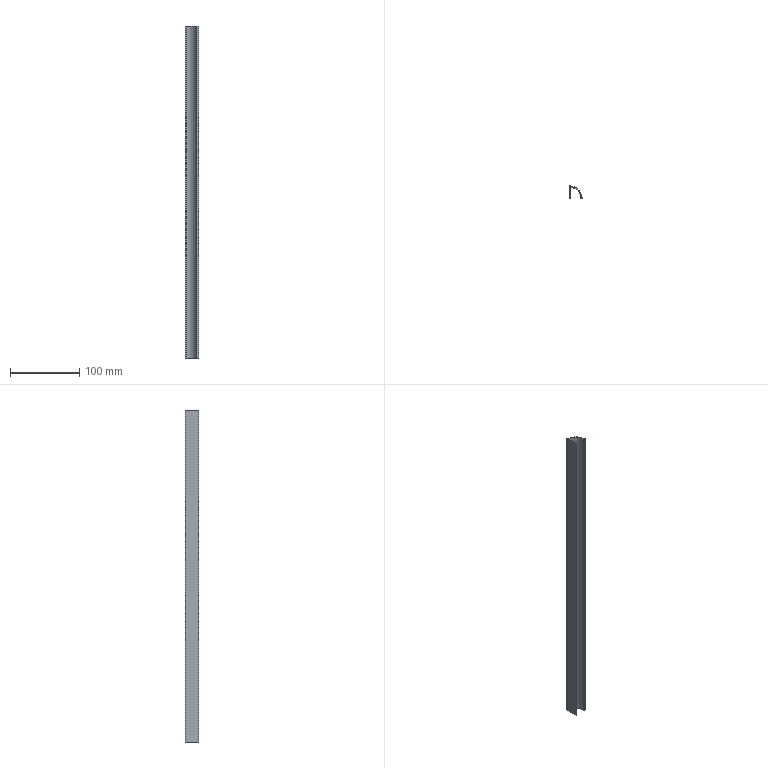Part | SolidWorks | features Extrusion 1 | 1 solid | 19 faces | box 19 x 19 x 480 mm | volume 26207 mm3 | plane 17 | cylinder 2 | commonest cylinder face diameters 30 x1 32 x1
STEP:
#1=CARTESIAN_POINT('',(0.,0.,0.));
#2=VERTEX_POINT('',#1);
#3=CARTESIAN_POINT('',(1.5,0.,0.));
#4=VERTEX_POINT('',#3);
#5=CARTESIAN_POINT('',(0.,0.,0.));
#6=DIRECTION('',(1.,0.,0.));
#7=VECTOR('',#6,1000.);
#8=LINE('',#5,#7);
#9=EDGE_CURVE('',#2,#4,#8,.T.);
#10=ORIENTED_EDGE('',*,*,#9,.T.);
#11=CARTESIAN_POINT('',(1.5,0.,480.));
#12=VERTEX_POINT('',#11);
#13=CARTESIAN_POINT('',(1.5,0.,480.));
#14=DIRECTION('',(0.,0.,-1.));
#15=VECTOR('',#14,1000.);
#16=LINE('',#13,#15);
#17=EDGE_CURVE('',#12,#4,#16,.T.);
#18=ORIENTED_EDGE('',*,*,#17,.F.);
#19=CARTESIAN_POINT('',(0.,0.,480.));
#20=VERTEX_POINT('',#19);
#21=CARTESIAN_POINT('',(0.,0.,480.));
#22=DIRECTION('',(1.,0.,0.));
#23=VECTOR('',#22,1000.);
#24=LINE('',#21,#23);
#25=EDGE_CURVE('',#20,#12,#24,.T.);
#26=ORIENTED_EDGE('',*,*,#25,.F.);
#27=CARTESIAN_POINT('',(0.,0.,480.));
#28=DIRECTION('',(0.,0.,-1.));
#29=VECTOR('',#28,1000.);
#30=LINE('',#27,#29);
#31=EDGE_CURVE('',#20,#2,#30,.T.);
#32=ORIENTED_EDGE('',*,*,#31,.T.);
#33=EDGE_LOOP('',(#10,#18,#26,#32));
#34=FACE_OUTER_BOUND('',#33,.T.);
#35=CARTESIAN_POINT('',(0.,0.,480.));
#36=DIRECTION('',(0.,1.,0.));
#37=DIRECTION('',(0.,0.,1.));
#38=AXIS2_PLACEMENT_3D('',#35,#36,#37);
#39=PLANE('',#38);
#40=ADVANCED_FACE('',(#34),#39,.F.);
#41=CARTESIAN_POINT('',(1.5,16.5,0.));
#42=VERTEX_POINT('',#41);
#43=CARTESIAN_POINT('',(1.5,0.,0.));
#44=DIRECTION('',(0.,1.,0.));
#45=VECTOR('',#44,1000.);
#46=LINE('',#43,#45);
#47=EDGE_CURVE('',#4,#42,#46,.T.);
#48=ORIENTED_EDGE('',*,*,#47,.T.);
#49=CARTESIAN_POINT('',(1.5,16.5,480.));
#50=VERTEX_POINT('',#49);
#51=CARTESIAN_POINT('',(1.5,16.5,480.));
#52=DIRECTION('',(0.,0.,-1.));
#53=VECTOR('',#52,1000.);
#54=LINE('',#51,#53);
#55=EDGE_CURVE('',#50,#42,#54,.T.);
#56=ORIENTED_EDGE('',*,*,#55,.F.);
#57=CARTESIAN_POINT('',(1.5,0.,480.));
#58=DIRECTION('',(0.,1.,0.));
#59=VECTOR('',#58,1000.);
#60=LINE('',#57,#59);
#61=EDGE_CURVE('',#12,#50,#60,.T.);
#62=ORIENTED_EDGE('',*,*,#61,.F.);
#63=ORIENTED_EDGE('',*,*,#17,.T.);
#64=EDGE_LOOP('',(#48,#56,#62,#63));
#65=FACE_OUTER_BOUND('',#64,.T.);
#66=CARTESIAN_POINT('',(1.5,0.,480.));
#67=DIRECTION('',(-1.,0.,0.));
#68=DIRECTION('',(0.,0.,1.));
#69=AXIS2_PLACEMENT_3D('',#66,#67,#68);
#70=PLANE('',#69);
#71=ADVANCED_FACE('',(#65),#70,.F.);
#72=CARTESIAN_POINT('',(16.5,1.5,0.));
#73=VERTEX_POINT('',#72);
#74=CARTESIAN_POINT('',(1.5,1.5,0.));
#75=DIRECTION('',(0.,0.,-1.));
#76=DIRECTION('',(-1.,0.,0.));
#77=AXIS2_PLACEMENT_3D('',#74,#75,#76);
#78=CIRCLE('',#77,15.);
#79=EDGE_CURVE('',#42,#73,#78,.T.);
#80=ORIENTED_EDGE('',*,*,#79,.T.);
#81=CARTESIAN_POINT('',(16.5,1.5,480.));
#82=VERTEX_POINT('',#81);
#83=CARTESIAN_POINT('',(16.5,1.5,480.));
#84=DIRECTION('',(0.,0.,-1.));
#85=VECTOR('',#84,1000.);
#86=LINE('',#83,#85);
#87=EDGE_CURVE('',#82,#73,#86,.T.);
#88=ORIENTED_EDGE('',*,*,#87,.F.);
#89=CARTESIAN_POINT('',(1.5,1.5,480.));
#90=DIRECTION('',(0.,0.,-1.));
#91=DIRECTION('',(-1.,0.,0.));
#92=AXIS2_PLACEMENT_3D('',#89,#90,#91);
#93=CIRCLE('',#92,15.);
#94=EDGE_CURVE('',#50,#82,#93,.T.);
#95=ORIENTED_EDGE('',*,*,#94,.F.);
#96=ORIENTED_EDGE('',*,*,#55,.T.);
#97=EDGE_LOOP('',(#80,#88,#95,#96));
#98=FACE_OUTER_BOUND('',#97,.T.);
#99=CARTESIAN_POINT('',(1.5,1.5,480.));
#100=DIRECTION('',(0.,0.,-1.));
#101=DIRECTION('',(-1.,0.,0.));
#102=AXIS2_PLACEMENT_3D('',#99,#100,#101);
#103=CYLINDRICAL_SURFACE('',#102,15.);
#104=ADVANCED_FACE('',(#98),#103,.F.);
#105=CARTESIAN_POINT('',(16.5,0.,0.));
#106=VERTEX_POINT('',#105);
#107=CARTESIAN_POINT('',(16.5,1.5,0.));
#108=DIRECTION('',(0.,-1.,0.));
#109=VECTOR('',#108,1000.);
#110=LINE('',#107,#109);
#111=EDGE_CURVE('',#73,#106,#110,.T.);
#112=ORIENTED_EDGE('',*,*,#111,.T.);
#113=CARTESIAN_POINT('',(16.5,0.,480.));
#114=VERTEX_POINT('',#113);
#115=CARTESIAN_POINT('',(16.5,0.,480.));
#116=DIRECTION('',(0.,0.,-1.));
#117=VECTOR('',#116,1000.);
#118=LINE('',#115,#117);
#119=EDGE_CURVE('',#114,#106,#118,.T.);
#120=ORIENTED_EDGE('',*,*,#119,.F.);
#121=CARTESIAN_POINT('',(16.5,1.5,480.));
#122=DIRECTION('',(0.,-1.,0.));
#123=VECTOR('',#122,1000.);
#124=LINE('',#121,#123);
#125=EDGE_CURVE('',#82,#114,#124,.T.);
#126=ORIENTED_EDGE('',*,*,#125,.F.);
#127=ORIENTED_EDGE('',*,*,#87,.T.);
#128=EDGE_LOOP('',(#112,#120,#126,#127));
#129=FACE_OUTER_BOUND('',#128,.T.);
#130=CARTESIAN_POINT('',(16.5,1.5,480.));
#131=DIRECTION('',(1.,0.,0.));
#132=DIRECTION('',(0.,0.,-1.));
#133=AXIS2_PLACEMENT_3D('',#130,#131,#132);
#134=PLANE('',#133);
#135=ADVANCED_FACE('',(#129),#134,.F.);
#136=CARTESIAN_POINT('',(19.,0.,0.));
#137=VERTEX_POINT('',#136);
#138=CARTESIAN_POINT('',(16.5,0.,0.));
#139=DIRECTION('',(1.,0.,0.));
#140=VECTOR('',#139,1000.);
#141=LINE('',#138,#140);
#142=EDGE_CURVE('',#106,#137,#141,.T.);
#143=ORIENTED_EDGE('',*,*,#142,.T.);
#144=CARTESIAN_POINT('',(19.,0.,480.));
#145=VERTEX_POINT('',#144);
#146=CARTESIAN_POINT('',(19.,0.,480.));
#147=DIRECTION('',(0.,0.,-1.));
#148=VECTOR('',#147,1000.);
#149=LINE('',#146,#148);
#150=EDGE_CURVE('',#145,#137,#149,.T.);
#151=ORIENTED_EDGE('',*,*,#150,.F.);
#152=CARTESIAN_POINT('',(16.5,0.,480.));
#153=DIRECTION('',(1.,0.,0.));
#154=VECTOR('',#153,1000.);
#155=LINE('',#152,#154);
#156=EDGE_CURVE('',#114,#145,#155,.T.);
#157=ORIENTED_EDGE('',*,*,#156,.F.);
#158=ORIENTED_EDGE('',*,*,#119,.T.);
#159=EDGE_LOOP('',(#143,#151,#157,#158));
#160=FACE_OUTER_BOUND('',#159,.T.);
#161=CARTESIAN_POINT('',(16.5,0.,480.));
#162=DIRECTION('',(0.,1.,0.));
#163=DIRECTION('',(0.,0.,1.));
#164=AXIS2_PLACEMENT_3D('',#161,#162,#163);
#165=PLANE('',#164);
#166=ADVANCED_FACE('',(#160),#165,.F.);
#167=CARTESIAN_POINT('',(19.,1.5,0.));
#168=VERTEX_POINT('',#167);
#169=CARTESIAN_POINT('',(19.,0.,0.));
#170=DIRECTION('',(0.,1.,0.));
#171=VECTOR('',#170,1000.);
#172=LINE('',#169,#171);
#173=EDGE_CURVE('',#137,#168,#172,.T.);
#174=ORIENTED_EDGE('',*,*,#173,.T.);
#175=CARTESIAN_POINT('',(19.,1.5,480.));
#176=VERTEX_POINT('',#175);
#177=CARTESIAN_POINT('',(19.,1.5,480.));
#178=DIRECTION('',(0.,0.,-1.));
#179=VECTOR('',#178,1000.);
#180=LINE('',#177,#179);
#181=EDGE_CURVE('',#176,#168,#180,.T.);
#182=ORIENTED_EDGE('',*,*,#181,.F.);
#183=CARTESIAN_POINT('',(19.,0.,480.));
#184=DIRECTION('',(0.,1.,0.));
#185=VECTOR('',#184,1000.);
#186=LINE('',#183,#185);
#187=EDGE_CURVE('',#145,#176,#186,.T.);
#188=ORIENTED_EDGE('',*,*,#187,.F.);
#189=ORIENTED_EDGE('',*,*,#150,.T.);
#190=EDGE_LOOP('',(#174,#182,#188,#189));
#191=FACE_OUTER_BOUND('',#190,.T.);
#192=CARTESIAN_POINT('',(19.,0.,480.));
#193=DIRECTION('',(-1.,0.,0.));
#194=DIRECTION('',(0.,0.,1.));
#195=AXIS2_PLACEMENT_3D('',#192,#193,#194);
#196=PLANE('',#195);
#197=ADVANCED_FACE('',(#191),#196,.F.);
#198=CARTESIAN_POINT('',(18.5,1.5,0.));
#199=VERTEX_POINT('',#198);
#200=CARTESIAN_POINT('',(18.5,1.5,0.));
#201=DIRECTION('',(-1.,0.,0.));
#202=VECTOR('',#201,1000.);
#203=LINE('',#200,#202);
#204=EDGE_CURVE('',#168,#199,#203,.T.);
#205=ORIENTED_EDGE('',*,*,#204,.T.);
#206=CARTESIAN_POINT('',(18.5,1.5,480.));
#207=VERTEX_POINT('',#206);
#208=CARTESIAN_POINT('',(18.5,1.5,480.));
#209=DIRECTION('',(0.,0.,-1.));
#210=VECTOR('',#209,1000.);
#211=LINE('',#208,#210);
#212=EDGE_CURVE('',#207,#199,#211,.T.);
#213=ORIENTED_EDGE('',*,*,#212,.F.);
#214=CARTESIAN_POINT('',(18.5,1.5,480.));
#215=DIRECTION('',(-1.,0.,0.));
#216=VECTOR('',#215,1000.);
#217=LINE('',#214,#216);
#218=EDGE_CURVE('',#176,#207,#217,.T.);
#219=ORIENTED_EDGE('',*,*,#218,.F.);
#220=ORIENTED_EDGE('',*,*,#181,.T.);
#221=EDGE_LOOP('',(#205,#213,#219,#220));
#222=FACE_OUTER_BOUND('',#221,.T.);
#223=CARTESIAN_POINT('',(18.5,1.5,480.));
#224=DIRECTION('',(0.,-1.,0.));
#225=DIRECTION('',(0.,0.,-1.));
#226=AXIS2_PLACEMENT_3D('',#223,#224,#225);
#227=PLANE('',#226);
#228=ADVANCED_FACE('',(#222),#227,.F.);
#229=CARTESIAN_POINT('',(18.5,0.5,0.));
#230=VERTEX_POINT('',#229);
#231=CARTESIAN_POINT('',(18.5,0.5,0.));
#232=DIRECTION('',(0.,-1.,0.));
#233=VECTOR('',#232,1000.);
#234=LINE('',#231,#233);
#235=EDGE_CURVE('',#199,#230,#234,.T.);
#236=ORIENTED_EDGE('',*,*,#235,.T.);
#237=CARTESIAN_POINT('',(18.5,0.5,480.));
#238=VERTEX_POINT('',#237);
#239=CARTESIAN_POINT('',(18.5,0.5,480.));
#240=DIRECTION('',(0.,0.,-1.));
#241=VECTOR('',#240,1000.);
#242=LINE('',#239,#241);
#243=EDGE_CURVE('',#238,#230,#242,.T.);
#244=ORIENTED_EDGE('',*,*,#243,.F.);
#245=CARTESIAN_POINT('',(18.5,0.5,480.));
#246=DIRECTION('',(0.,-1.,0.));
#247=VECTOR('',#246,1000.);
#248=LINE('',#245,#247);
#249=EDGE_CURVE('',#207,#238,#248,.T.);
#250=ORIENTED_EDGE('',*,*,#249,.F.);
#251=ORIENTED_EDGE('',*,*,#212,.T.);
#252=EDGE_LOOP('',(#236,#244,#250,#251));
#253=FACE_OUTER_BOUND('',#252,.T.);
#254=CARTESIAN_POINT('',(18.5,0.5,480.));
#255=DIRECTION('',(1.,0.,0.));
#256=DIRECTION('',(0.,0.,-1.));
#257=AXIS2_PLACEMENT_3D('',#254,#255,#256);
#258=PLANE('',#257);
#259=ADVANCED_FACE('',(#253),#258,.F.);
#260=CARTESIAN_POINT('',(17.5,0.5,0.));
#261=VERTEX_POINT('',#260);
#262=CARTESIAN_POINT('',(17.5,0.5,0.));
#263=DIRECTION('',(-1.,0.,0.));
#264=VECTOR('',#263,1000.);
#265=LINE('',#262,#264);
#266=EDGE_CURVE('',#230,#261,#265,.T.);
#267=ORIENTED_EDGE('',*,*,#266,.T.);
#268=CARTESIAN_POINT('',(17.5,0.5,480.));
#269=VERTEX_POINT('',#268);
#270=CARTESIAN_POINT('',(17.5,0.5,480.));
#271=DIRECTION('',(0.,0.,-1.));
#272=VECTOR('',#271,1000.);
#273=LINE('',#270,#272);
#274=EDGE_CURVE('',#269,#261,#273,.T.);
#275=ORIENTED_EDGE('',*,*,#274,.F.);
#276=CARTESIAN_POINT('',(17.5,0.5,480.));
#277=DIRECTION('',(-1.,0.,0.));
#278=VECTOR('',#277,1000.);
#279=LINE('',#276,#278);
#280=EDGE_CURVE('',#238,#269,#279,.T.);
#281=ORIENTED_EDGE('',*,*,#280,.F.);
#282=ORIENTED_EDGE('',*,*,#243,.T.);
#283=EDGE_LOOP('',(#267,#275,#281,#282));
#284=FACE_OUTER_BOUND('',#283,.T.);
#285=CARTESIAN_POINT('',(17.5,0.5,480.));
#286=DIRECTION('',(0.,-1.,0.));
#287=DIRECTION('',(0.,0.,-1.));
#288=AXIS2_PLACEMENT_3D('',#285,#286,#287);
#289=PLANE('',#288);
#290=ADVANCED_FACE('',(#284),#289,.F.);
#291=CARTESIAN_POINT('',(17.5,1.5,0.));
#292=VERTEX_POINT('',#291);
#293=CARTESIAN_POINT('',(17.5,1.5,0.));
#294=DIRECTION('',(0.,1.,0.));
#295=VECTOR('',#294,1000.);
#296=LINE('',#293,#295);
#297=EDGE_CURVE('',#261,#292,#296,.T.);
#298=ORIENTED_EDGE('',*,*,#297,.T.);
#299=CARTESIAN_POINT('',(17.5,1.5,480.));
#300=VERTEX_POINT('',#299);
#301=CARTESIAN_POINT('',(17.5,1.5,480.));
#302=DIRECTION('',(0.,0.,-1.));
#303=VECTOR('',#302,1000.);
#304=LINE('',#301,#303);
#305=EDGE_CURVE('',#300,#292,#304,.T.);
#306=ORIENTED_EDGE('',*,*,#305,.F.);
#307=CARTESIAN_POINT('',(17.5,1.5,480.));
#308=DIRECTION('',(0.,1.,0.));
#309=VECTOR('',#308,1000.);
#310=LINE('',#307,#309);
#311=EDGE_CURVE('',#269,#300,#310,.T.);
#312=ORIENTED_EDGE('',*,*,#311,.F.);
#313=ORIENTED_EDGE('',*,*,#274,.T.);
#314=EDGE_LOOP('',(#298,#306,#312,#313));
#315=FACE_OUTER_BOUND('',#314,.T.);
#316=CARTESIAN_POINT('',(17.5,1.5,480.));
#317=DIRECTION('',(-1.,0.,0.));
#318=DIRECTION('',(0.,0.,1.));
#319=AXIS2_PLACEMENT_3D('',#316,#317,#318);
#320=PLANE('',#319);
#321=ADVANCED_FACE('',(#315),#320,.F.);
#322=CARTESIAN_POINT('',(1.5,17.5,0.));
#323=VERTEX_POINT('',#322);
#324=CARTESIAN_POINT('',(1.5,1.5,0.));
#325=DIRECTION('',(0.,0.,1.));
#326=DIRECTION('',(-1.,0.,0.));
#327=AXIS2_PLACEMENT_3D('',#324,#325,#326);
#328=CIRCLE('',#327,16.);
#329=EDGE_CURVE('',#292,#323,#328,.T.);
#330=ORIENTED_EDGE('',*,*,#329,.T.);
#331=CARTESIAN_POINT('',(1.5,17.5,480.));
#332=VERTEX_POINT('',#331);
#333=CARTESIAN_POINT('',(1.5,17.5,480.));
#334=DIRECTION('',(0.,0.,-1.));
#335=VECTOR('',#334,1000.);
#336=LINE('',#333,#335);
#337=EDGE_CURVE('',#332,#323,#336,.T.);
#338=ORIENTED_EDGE('',*,*,#337,.F.);
#339=CARTESIAN_POINT('',(1.5,1.5,480.));
#340=DIRECTION('',(0.,0.,1.));
#341=DIRECTION('',(-1.,0.,0.));
#342=AXIS2_PLACEMENT_3D('',#339,#340,#341);
#343=CIRCLE('',#342,16.);
#344=EDGE_CURVE('',#300,#332,#343,.T.);
#345=ORIENTED_EDGE('',*,*,#344,.F.);
#346=ORIENTED_EDGE('',*,*,#305,.T.);
#347=EDGE_LOOP('',(#330,#338,#345,#346));
#348=FACE_OUTER_BOUND('',#347,.T.);
#349=CARTESIAN_POINT('',(1.5,1.5,480.));
#350=DIRECTION('',(0.,0.,-1.));
#351=DIRECTION('',(-1.,0.,0.));
#352=AXIS2_PLACEMENT_3D('',#349,#350,#351);
#353=CYLINDRICAL_SURFACE('',#352,16.);
#354=ADVANCED_FACE('',(#348),#353,.T.);
#355=CARTESIAN_POINT('',(0.5,17.5,0.));
#356=VERTEX_POINT('',#355);
#357=CARTESIAN_POINT('',(0.5,17.5,0.));
#358=DIRECTION('',(-1.,0.,0.));
#359=VECTOR('',#358,1000.);
#360=LINE('',#357,#359);
#361=EDGE_CURVE('',#323,#356,#360,.T.);
#362=ORIENTED_EDGE('',*,*,#361,.T.);
#363=CARTESIAN_POINT('',(0.5,17.5,480.));
#364=VERTEX_POINT('',#363);
#365=CARTESIAN_POINT('',(0.5,17.5,480.));
#366=DIRECTION('',(0.,0.,-1.));
#367=VECTOR('',#366,1000.);
#368=LINE('',#365,#367);
#369=EDGE_CURVE('',#364,#356,#368,.T.);
#370=ORIENTED_EDGE('',*,*,#369,.F.);
#371=CARTESIAN_POINT('',(0.5,17.5,480.));
#372=DIRECTION('',(-1.,0.,0.));
#373=VECTOR('',#372,1000.);
#374=LINE('',#371,#373);
#375=EDGE_CURVE('',#332,#364,#374,.T.);
#376=ORIENTED_EDGE('',*,*,#375,.F.);
#377=ORIENTED_EDGE('',*,*,#337,.T.);
#378=EDGE_LOOP('',(#362,#370,#376,#377));
#379=FACE_OUTER_BOUND('',#378,.T.);
#380=CARTESIAN_POINT('',(0.5,17.5,480.));
#381=DIRECTION('',(0.,-1.,0.));
#382=DIRECTION('',(0.,0.,-1.));
#383=AXIS2_PLACEMENT_3D('',#380,#381,#382);
#384=PLANE('',#383);
#385=ADVANCED_FACE('',(#379),#384,.F.);
#386=CARTESIAN_POINT('',(0.5,18.5,0.));
#387=VERTEX_POINT('',#386);
#388=CARTESIAN_POINT('',(0.5,18.5,0.));
#389=DIRECTION('',(0.,1.,0.));
#390=VECTOR('',#389,1000.);
#391=LINE('',#388,#390);
#392=EDGE_CURVE('',#356,#387,#391,.T.);
#393=ORIENTED_EDGE('',*,*,#392,.T.);
#394=CARTESIAN_POINT('',(0.5,18.5,480.));
#395=VERTEX_POINT('',#394);
#396=CARTESIAN_POINT('',(0.5,18.5,480.));
#397=DIRECTION('',(0.,0.,-1.));
#398=VECTOR('',#397,1000.);
#399=LINE('',#396,#398);
#400=EDGE_CURVE('',#395,#387,#399,.T.);
#401=ORIENTED_EDGE('',*,*,#400,.F.);
#402=CARTESIAN_POINT('',(0.5,18.5,480.));
#403=DIRECTION('',(0.,1.,0.));
#404=VECTOR('',#403,1000.);
#405=LINE('',#402,#404);
#406=EDGE_CURVE('',#364,#395,#405,.T.);
#407=ORIENTED_EDGE('',*,*,#406,.F.);
#408=ORIENTED_EDGE('',*,*,#369,.T.);
#409=EDGE_LOOP('',(#393,#401,#407,#408));
#410=FACE_OUTER_BOUND('',#409,.T.);
#411=CARTESIAN_POINT('',(0.5,18.5,480.));
#412=DIRECTION('',(-1.,0.,0.));
#413=DIRECTION('',(0.,0.,1.));
#414=AXIS2_PLACEMENT_3D('',#411,#412,#413);
#415=PLANE('',#414);
#416=ADVANCED_FACE('',(#410),#415,.F.);
#417=CARTESIAN_POINT('',(1.5,18.5,0.));
#418=VERTEX_POINT('',#417);
#419=CARTESIAN_POINT('',(1.5,18.5,0.));
#420=DIRECTION('',(1.,0.,0.));
#421=VECTOR('',#420,1000.);
#422=LINE('',#419,#421);
#423=EDGE_CURVE('',#387,#418,#422,.T.);
#424=ORIENTED_EDGE('',*,*,#423,.T.);
#425=CARTESIAN_POINT('',(1.5,18.5,480.));
#426=VERTEX_POINT('',#425);
#427=CARTESIAN_POINT('',(1.5,18.5,480.));
#428=DIRECTION('',(0.,0.,-1.));
#429=VECTOR('',#428,1000.);
#430=LINE('',#427,#429);
#431=EDGE_CURVE('',#426,#418,#430,.T.);
#432=ORIENTED_EDGE('',*,*,#431,.F.);
#433=CARTESIAN_POINT('',(1.5,18.5,480.));
#434=DIRECTION('',(1.,0.,0.));
#435=VECTOR('',#434,1000.);
#436=LINE('',#433,#435);
#437=EDGE_CURVE('',#395,#426,#436,.T.);
#438=ORIENTED_EDGE('',*,*,#437,.F.);
#439=ORIENTED_EDGE('',*,*,#400,.T.);
#440=EDGE_LOOP('',(#424,#432,#438,#439));
#441=FACE_OUTER_BOUND('',#440,.T.);
#442=CARTESIAN_POINT('',(1.5,18.5,480.));
#443=DIRECTION('',(0.,1.,0.));
#444=DIRECTION('',(0.,0.,1.));
#445=AXIS2_PLACEMENT_3D('',#442,#443,#444);
#446=PLANE('',#445);
#447=ADVANCED_FACE('',(#441),#446,.F.);
#448=CARTESIAN_POINT('',(1.5,19.,0.));
#449=VERTEX_POINT('',#448);
#450=CARTESIAN_POINT('',(1.5,19.,0.));
#451=DIRECTION('',(0.,1.,0.));
#452=VECTOR('',#451,1000.);
#453=LINE('',#450,#452);
#454=EDGE_CURVE('',#418,#449,#453,.T.);
#455=ORIENTED_EDGE('',*,*,#454,.T.);
#456=CARTESIAN_POINT('',(1.5,19.,480.));
#457=VERTEX_POINT('',#456);
#458=CARTESIAN_POINT('',(1.5,19.,480.));
#459=DIRECTION('',(0.,0.,-1.));
#460=VECTOR('',#459,1000.);
#461=LINE('',#458,#460);
#462=EDGE_CURVE('',#457,#449,#461,.T.);
#463=ORIENTED_EDGE('',*,*,#462,.F.);
#464=CARTESIAN_POINT('',(1.5,19.,480.));
#465=DIRECTION('',(0.,1.,0.));
#466=VECTOR('',#465,1000.);
#467=LINE('',#464,#466);
#468=EDGE_CURVE('',#426,#457,#467,.T.);
#469=ORIENTED_EDGE('',*,*,#468,.F.);
#470=ORIENTED_EDGE('',*,*,#431,.T.);
#471=EDGE_LOOP('',(#455,#463,#469,#470));
#472=FACE_OUTER_BOUND('',#471,.T.);
#473=CARTESIAN_POINT('',(1.5,19.,480.));
#474=DIRECTION('',(-1.,0.,0.));
#475=DIRECTION('',(0.,0.,1.));
#476=AXIS2_PLACEMENT_3D('',#473,#474,#475);
#477=PLANE('',#476);
#478=ADVANCED_FACE('',(#472),#477,.F.);
#479=CARTESIAN_POINT('',(0.,19.,0.));
#480=VERTEX_POINT('',#479);
#481=CARTESIAN_POINT('',(0.,19.,0.));
#482=DIRECTION('',(-1.,0.,0.));
#483=VECTOR('',#482,1000.);
#484=LINE('',#481,#483);
#485=EDGE_CURVE('',#449,#480,#484,.T.);
#486=ORIENTED_EDGE('',*,*,#485,.T.);
#487=CARTESIAN_POINT('',(0.,19.,480.));
#488=VERTEX_POINT('',#487);
#489=CARTESIAN_POINT('',(0.,19.,480.));
#490=DIRECTION('',(0.,0.,-1.));
#491=VECTOR('',#490,1000.);
#492=LINE('',#489,#491);
#493=EDGE_CURVE('',#488,#480,#492,.T.);
#494=ORIENTED_EDGE('',*,*,#493,.F.);
#495=CARTESIAN_POINT('',(0.,19.,480.));
#496=DIRECTION('',(-1.,0.,0.));
#497=VECTOR('',#496,1000.);
#498=LINE('',#495,#497);
#499=EDGE_CURVE('',#457,#488,#498,.T.);
#500=ORIENTED_EDGE('',*,*,#499,.F.);
#501=ORIENTED_EDGE('',*,*,#462,.T.);
#502=EDGE_LOOP('',(#486,#494,#500,#501));
#503=FACE_OUTER_BOUND('',#502,.T.);
#504=CARTESIAN_POINT('',(0.,19.,480.));
#505=DIRECTION('',(0.,-1.,0.));
#506=DIRECTION('',(0.,0.,-1.));
#507=AXIS2_PLACEMENT_3D('',#504,#505,#506);
#508=PLANE('',#507);
#509=ADVANCED_FACE('',(#503),#508,.F.);
#510=CARTESIAN_POINT('',(0.,0.,0.));
#511=DIRECTION('',(0.,-1.,0.));
#512=VECTOR('',#511,1000.);
#513=LINE('',#510,#512);
#514=EDGE_CURVE('',#480,#2,#513,.T.);
#515=ORIENTED_EDGE('',*,*,#514,.T.);
#516=ORIENTED_EDGE('',*,*,#31,.F.);
#517=CARTESIAN_POINT('',(0.,0.,480.));
#518=DIRECTION('',(0.,-1.,0.));
#519=VECTOR('',#518,1000.);
#520=LINE('',#517,#519);
#521=EDGE_CURVE('',#488,#20,#520,.T.);
#522=ORIENTED_EDGE('',*,*,#521,.F.);
#523=ORIENTED_EDGE('',*,*,#493,.T.);
#524=EDGE_LOOP('',(#515,#516,#522,#523));
#525=FACE_OUTER_BOUND('',#524,.T.);
#526=CARTESIAN_POINT('',(0.,0.,480.));
#527=DIRECTION('',(1.,0.,0.));
#528=DIRECTION('',(0.,0.,-1.));
#529=AXIS2_PLACEMENT_3D('',#526,#527,#528);
#530=PLANE('',#529);
#531=ADVANCED_FACE('',(#525),#530,.F.);
#532=ORIENTED_EDGE('',*,*,#25,.T.);
#533=ORIENTED_EDGE('',*,*,#61,.T.);
#534=ORIENTED_EDGE('',*,*,#94,.T.);
#535=ORIENTED_EDGE('',*,*,#125,.T.);
#536=ORIENTED_EDGE('',*,*,#156,.T.);
#537=ORIENTED_EDGE('',*,*,#187,.T.);
#538=ORIENTED_EDGE('',*,*,#218,.T.);
#539=ORIENTED_EDGE('',*,*,#249,.T.);
#540=ORIENTED_EDGE('',*,*,#280,.T.);
#541=ORIENTED_EDGE('',*,*,#311,.T.);
#542=ORIENTED_EDGE('',*,*,#344,.T.);
#543=ORIENTED_EDGE('',*,*,#375,.T.);
#544=ORIENTED_EDGE('',*,*,#406,.T.);
#545=ORIENTED_EDGE('',*,*,#437,.T.);
#546=ORIENTED_EDGE('',*,*,#468,.T.);
#547=ORIENTED_EDGE('',*,*,#499,.T.);
#548=ORIENTED_EDGE('',*,*,#521,.T.);
#549=EDGE_LOOP('',(#532,#533,#534,#535,#536,#537,#538,#539,#540,#541,#542,#543,#544,#545,#546,#547,#548));
#550=FACE_OUTER_BOUND('',#549,.T.);
#551=CARTESIAN_POINT('',(1.5,1.5,480.));
#552=DIRECTION('',(0.,0.,-1.));
#553=DIRECTION('',(-1.,0.,0.));
#554=AXIS2_PLACEMENT_3D('',#551,#552,#553);
#555=PLANE('',#554);
#556=ADVANCED_FACE('',(#550),#555,.F.);
#557=ORIENTED_EDGE('',*,*,#9,.F.);
#558=ORIENTED_EDGE('',*,*,#514,.F.);
#559=ORIENTED_EDGE('',*,*,#485,.F.);
#560=ORIENTED_EDGE('',*,*,#454,.F.);
#561=ORIENTED_EDGE('',*,*,#423,.F.);
#562=ORIENTED_EDGE('',*,*,#392,.F.);
#563=ORIENTED_EDGE('',*,*,#361,.F.);
#564=ORIENTED_EDGE('',*,*,#329,.F.);
#565=ORIENTED_EDGE('',*,*,#297,.F.);
#566=ORIENTED_EDGE('',*,*,#266,.F.);
#567=ORIENTED_EDGE('',*,*,#235,.F.);
#568=ORIENTED_EDGE('',*,*,#204,.F.);
#569=ORIENTED_EDGE('',*,*,#173,.F.);
#570=ORIENTED_EDGE('',*,*,#142,.F.);
#571=ORIENTED_EDGE('',*,*,#111,.F.);
#572=ORIENTED_EDGE('',*,*,#79,.F.);
#573=ORIENTED_EDGE('',*,*,#47,.F.);
#574=EDGE_LOOP('',(#557,#558,#559,#560,#561,#562,#563,#564,#565,#566,#567,#568,#569,#570,#571,#572,#573));
#575=FACE_OUTER_BOUND('',#574,.T.);
#576=CARTESIAN_POINT('',(1.5,1.5,0.));
#577=DIRECTION('',(0.,0.,-1.));
#578=DIRECTION('',(-1.,0.,0.));
#579=AXIS2_PLACEMENT_3D('',#576,#577,#578);
#580=PLANE('',#579);
#581=ADVANCED_FACE('',(#575),#580,.T.);
#582=CLOSED_SHELL('',(#40,#71,#104,#135,#166,#197,#228,#259,#290,#321,#354,#385,#416,#447,#478,#509,#531,#556,#581));
#583=MANIFOLD_SOLID_BREP('',#582);
#584=CARTESIAN_POINT('',(0.,0.,0.));
#585=DIRECTION('',(0.,0.,1.));
#586=DIRECTION('',(1.,0.,0.));
#587=AXIS2_PLACEMENT_3D('',#584,#585,#586);
#588=(LENGTH_UNIT()NAMED_UNIT(*)SI_UNIT(.MILLI.,.METRE.));
#589=UNCERTAINTY_MEASURE_WITH_UNIT(LENGTH_MEASURE(0.00001),#588,'','');
#590=(NAMED_UNIT(*)PLANE_ANGLE_UNIT()SI_UNIT($,.RADIAN.));
#591=(NAMED_UNIT(*)SI_UNIT($,.STERADIAN.)SOLID_ANGLE_UNIT());
#592=(GEOMETRIC_REPRESENTATION_CONTEXT(3)GLOBAL_UNCERTAINTY_ASSIGNED_CONTEXT((#589))GLOBAL_UNIT_ASSIGNED_CONTEXT((#588,#590,#591))REPRESENTATION_CONTEXT('',''));
#593=ADVANCED_BREP_SHAPE_REPRESENTATION('',(#583,#587),#592);